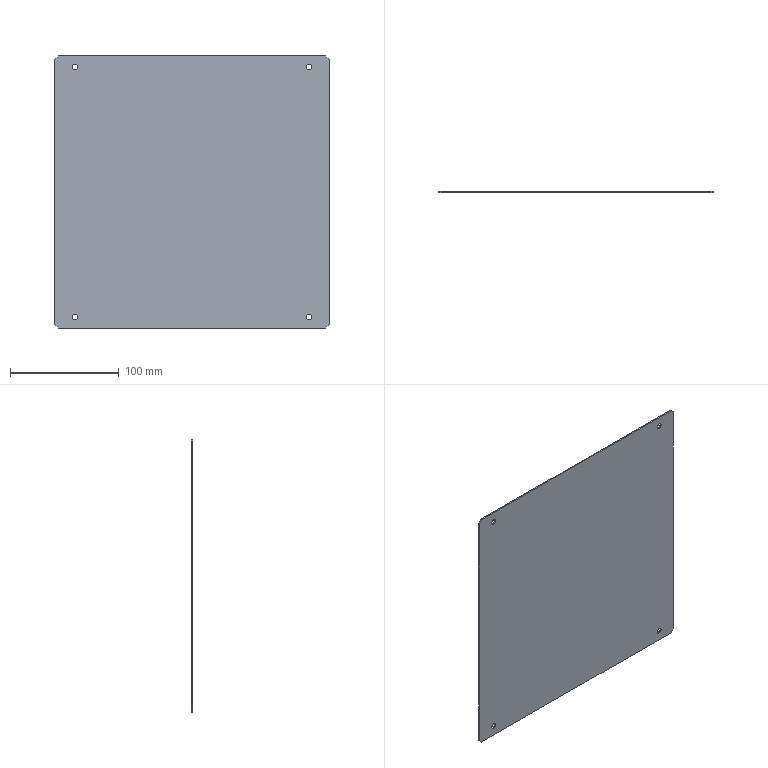Part | STEP file | 1519D3-3_AF0.stp.STEP | 1 solid | 18 faces | box 252 x 1.2 x 250 mm | volume 75484 mm3 | plane 10 | cylinder 8 | commonest cylinder face diameters 5 x8
STEP:
#1=CARTESIAN_POINT('',(105.,0.,-115.));
#2=VERTEX_POINT('',#1);
#3=CARTESIAN_POINT('',(110.,0.,-115.));
#4=VERTEX_POINT('',#3);
#5=CARTESIAN_POINT('',(107.5,0.,-115.));
#6=DIRECTION('',(0.,1.,0.));
#7=DIRECTION('',(-1.,0.,0.));
#8=AXIS2_PLACEMENT_3D('',#5,#6,#7);
#9=CIRCLE('',#8,2.5);
#10=EDGE_CURVE('',#2,#4,#9,.T.);
#11=ORIENTED_EDGE('',*,*,#10,.T.);
#12=CARTESIAN_POINT('',(107.5,0.,-115.));
#13=DIRECTION('',(0.,1.,0.));
#14=DIRECTION('',(1.,0.,0.));
#15=AXIS2_PLACEMENT_3D('',#12,#13,#14);
#16=CIRCLE('',#15,2.5);
#17=EDGE_CURVE('',#4,#2,#16,.T.);
#18=ORIENTED_EDGE('',*,*,#17,.T.);
#19=EDGE_LOOP('',(#11,#18));
#20=FACE_BOUND('',#19,.T.);
#21=CARTESIAN_POINT('',(105.,0.,115.));
#22=VERTEX_POINT('',#21);
#23=CARTESIAN_POINT('',(110.,0.,115.));
#24=VERTEX_POINT('',#23);
#25=CARTESIAN_POINT('',(107.5,0.,115.));
#26=DIRECTION('',(0.,1.,0.));
#27=DIRECTION('',(-1.,0.,0.));
#28=AXIS2_PLACEMENT_3D('',#25,#26,#27);
#29=CIRCLE('',#28,2.5);
#30=EDGE_CURVE('',#22,#24,#29,.T.);
#31=ORIENTED_EDGE('',*,*,#30,.T.);
#32=CARTESIAN_POINT('',(107.5,0.,115.));
#33=DIRECTION('',(0.,1.,0.));
#34=DIRECTION('',(1.,0.,0.));
#35=AXIS2_PLACEMENT_3D('',#32,#33,#34);
#36=CIRCLE('',#35,2.5);
#37=EDGE_CURVE('',#24,#22,#36,.T.);
#38=ORIENTED_EDGE('',*,*,#37,.T.);
#39=EDGE_LOOP('',(#31,#38));
#40=FACE_BOUND('',#39,.T.);
#41=CARTESIAN_POINT('',(-110.,0.,115.));
#42=VERTEX_POINT('',#41);
#43=CARTESIAN_POINT('',(-105.,0.,115.));
#44=VERTEX_POINT('',#43);
#45=CARTESIAN_POINT('',(-107.5,0.,115.));
#46=DIRECTION('',(0.,1.,0.));
#47=DIRECTION('',(-1.,0.,0.));
#48=AXIS2_PLACEMENT_3D('',#45,#46,#47);
#49=CIRCLE('',#48,2.5);
#50=EDGE_CURVE('',#42,#44,#49,.T.);
#51=ORIENTED_EDGE('',*,*,#50,.T.);
#52=CARTESIAN_POINT('',(-107.5,0.,115.));
#53=DIRECTION('',(0.,1.,0.));
#54=DIRECTION('',(1.,0.,0.));
#55=AXIS2_PLACEMENT_3D('',#52,#53,#54);
#56=CIRCLE('',#55,2.5);
#57=EDGE_CURVE('',#44,#42,#56,.T.);
#58=ORIENTED_EDGE('',*,*,#57,.T.);
#59=EDGE_LOOP('',(#51,#58));
#60=FACE_BOUND('',#59,.T.);
#61=CARTESIAN_POINT('',(-110.,0.,-115.));
#62=VERTEX_POINT('',#61);
#63=CARTESIAN_POINT('',(-105.,0.,-115.));
#64=VERTEX_POINT('',#63);
#65=CARTESIAN_POINT('',(-107.5,0.,-115.));
#66=DIRECTION('',(0.,1.,0.));
#67=DIRECTION('',(-1.,0.,0.));
#68=AXIS2_PLACEMENT_3D('',#65,#66,#67);
#69=CIRCLE('',#68,2.5);
#70=EDGE_CURVE('',#62,#64,#69,.T.);
#71=ORIENTED_EDGE('',*,*,#70,.T.);
#72=CARTESIAN_POINT('',(-107.5,0.,-115.));
#73=DIRECTION('',(0.,1.,0.));
#74=DIRECTION('',(1.,0.,0.));
#75=AXIS2_PLACEMENT_3D('',#72,#73,#74);
#76=CIRCLE('',#75,2.5);
#77=EDGE_CURVE('',#64,#62,#76,.T.);
#78=ORIENTED_EDGE('',*,*,#77,.T.);
#79=EDGE_LOOP('',(#71,#78));
#80=FACE_BOUND('',#79,.T.);
#81=CARTESIAN_POINT('',(123.,0.,-125.));
#82=VERTEX_POINT('',#81);
#83=CARTESIAN_POINT('',(-123.,0.,-125.));
#84=VERTEX_POINT('',#83);
#85=CARTESIAN_POINT('',(123.,0.,-125.));
#86=DIRECTION('',(-1.,0.,0.));
#87=VECTOR('',#86,1000.);
#88=LINE('',#85,#87);
#89=EDGE_CURVE('',#82,#84,#88,.T.);
#90=ORIENTED_EDGE('',*,*,#89,.F.);
#91=CARTESIAN_POINT('',(126.,0.,-122.));
#92=VERTEX_POINT('',#91);
#93=CARTESIAN_POINT('',(123.,0.,-125.));
#94=DIRECTION('',(0.7071,0.,0.7071));
#95=VECTOR('',#94,1000.);
#96=LINE('',#93,#95);
#97=EDGE_CURVE('',#82,#92,#96,.T.);
#98=ORIENTED_EDGE('',*,*,#97,.T.);
#99=CARTESIAN_POINT('',(126.,0.,122.));
#100=VERTEX_POINT('',#99);
#101=CARTESIAN_POINT('',(126.,0.,122.));
#102=DIRECTION('',(0.,0.,-1.));
#103=VECTOR('',#102,1000.);
#104=LINE('',#101,#103);
#105=EDGE_CURVE('',#100,#92,#104,.T.);
#106=ORIENTED_EDGE('',*,*,#105,.F.);
#107=CARTESIAN_POINT('',(123.,0.,125.));
#108=VERTEX_POINT('',#107);
#109=CARTESIAN_POINT('',(126.,0.,122.));
#110=DIRECTION('',(-0.7071,0.,0.7071));
#111=VECTOR('',#110,1000.);
#112=LINE('',#109,#111);
#113=EDGE_CURVE('',#100,#108,#112,.T.);
#114=ORIENTED_EDGE('',*,*,#113,.T.);
#115=CARTESIAN_POINT('',(-123.,0.,125.));
#116=VERTEX_POINT('',#115);
#117=CARTESIAN_POINT('',(-123.,0.,125.));
#118=DIRECTION('',(1.,0.,0.));
#119=VECTOR('',#118,1000.);
#120=LINE('',#117,#119);
#121=EDGE_CURVE('',#116,#108,#120,.T.);
#122=ORIENTED_EDGE('',*,*,#121,.F.);
#123=CARTESIAN_POINT('',(-126.,0.,122.));
#124=VERTEX_POINT('',#123);
#125=CARTESIAN_POINT('',(-123.,0.,125.));
#126=DIRECTION('',(-0.7071,0.,-0.7071));
#127=VECTOR('',#126,1000.);
#128=LINE('',#125,#127);
#129=EDGE_CURVE('',#116,#124,#128,.T.);
#130=ORIENTED_EDGE('',*,*,#129,.T.);
#131=CARTESIAN_POINT('',(-126.,0.,-122.));
#132=VERTEX_POINT('',#131);
#133=CARTESIAN_POINT('',(-126.,0.,-122.));
#134=DIRECTION('',(0.,0.,1.));
#135=VECTOR('',#134,1000.);
#136=LINE('',#133,#135);
#137=EDGE_CURVE('',#132,#124,#136,.T.);
#138=ORIENTED_EDGE('',*,*,#137,.F.);
#139=CARTESIAN_POINT('',(-126.,0.,-122.));
#140=DIRECTION('',(0.7071,0.,-0.7071));
#141=VECTOR('',#140,1000.);
#142=LINE('',#139,#141);
#143=EDGE_CURVE('',#132,#84,#142,.T.);
#144=ORIENTED_EDGE('',*,*,#143,.T.);
#145=EDGE_LOOP('',(#90,#98,#106,#114,#122,#130,#138,#144));
#146=FACE_OUTER_BOUND('',#145,.T.);
#147=CARTESIAN_POINT('',(0.,0.,0.));
#148=DIRECTION('',(0.,1.,0.));
#149=DIRECTION('',(1.,0.,0.));
#150=AXIS2_PLACEMENT_3D('',#147,#148,#149);
#151=PLANE('',#150);
#152=ADVANCED_FACE('',(#20,#40,#60,#80,#146),#151,.F.);
#153=CARTESIAN_POINT('',(-105.,1.2,-115.));
#154=VERTEX_POINT('',#153);
#155=CARTESIAN_POINT('',(-105.,1.2,-115.));
#156=DIRECTION('',(0.,-1.,0.));
#157=VECTOR('',#156,1000.);
#158=LINE('',#155,#157);
#159=EDGE_CURVE('',#154,#64,#158,.T.);
#160=ORIENTED_EDGE('',*,*,#159,.F.);
#161=CARTESIAN_POINT('',(-110.,1.2,-115.));
#162=VERTEX_POINT('',#161);
#163=CARTESIAN_POINT('',(-107.5,1.2,-115.));
#164=DIRECTION('',(0.,1.,0.));
#165=DIRECTION('',(1.,0.,0.));
#166=AXIS2_PLACEMENT_3D('',#163,#164,#165);
#167=CIRCLE('',#166,2.5);
#168=EDGE_CURVE('',#154,#162,#167,.T.);
#169=ORIENTED_EDGE('',*,*,#168,.T.);
#170=CARTESIAN_POINT('',(-110.,1.2,-115.));
#171=DIRECTION('',(0.,-1.,0.));
#172=VECTOR('',#171,1000.);
#173=LINE('',#170,#172);
#174=EDGE_CURVE('',#162,#62,#173,.T.);
#175=ORIENTED_EDGE('',*,*,#174,.T.);
#176=ORIENTED_EDGE('',*,*,#77,.F.);
#177=EDGE_LOOP('',(#160,#169,#175,#176));
#178=FACE_OUTER_BOUND('',#177,.T.);
#179=CARTESIAN_POINT('',(-107.5,1.2,-115.));
#180=DIRECTION('',(0.,1.,0.));
#181=DIRECTION('',(1.,0.,0.));
#182=AXIS2_PLACEMENT_3D('',#179,#180,#181);
#183=CYLINDRICAL_SURFACE('',#182,2.5);
#184=ADVANCED_FACE('',(#178),#183,.F.);
#185=ORIENTED_EDGE('',*,*,#174,.F.);
#186=CARTESIAN_POINT('',(-107.5,1.2,-115.));
#187=DIRECTION('',(0.,1.,0.));
#188=DIRECTION('',(-1.,0.,0.));
#189=AXIS2_PLACEMENT_3D('',#186,#187,#188);
#190=CIRCLE('',#189,2.5);
#191=EDGE_CURVE('',#162,#154,#190,.T.);
#192=ORIENTED_EDGE('',*,*,#191,.T.);
#193=ORIENTED_EDGE('',*,*,#159,.T.);
#194=ORIENTED_EDGE('',*,*,#70,.F.);
#195=EDGE_LOOP('',(#185,#192,#193,#194));
#196=FACE_OUTER_BOUND('',#195,.T.);
#197=CARTESIAN_POINT('',(-107.5,1.2,-115.));
#198=DIRECTION('',(0.,1.,0.));
#199=DIRECTION('',(1.,0.,0.));
#200=AXIS2_PLACEMENT_3D('',#197,#198,#199);
#201=CYLINDRICAL_SURFACE('',#200,2.5);
#202=ADVANCED_FACE('',(#196),#201,.F.);
#203=CARTESIAN_POINT('',(105.,1.2,-115.));
#204=VERTEX_POINT('',#203);
#205=CARTESIAN_POINT('',(110.,1.2,-115.));
#206=VERTEX_POINT('',#205);
#207=CARTESIAN_POINT('',(107.5,1.2,-115.));
#208=DIRECTION('',(0.,1.,0.));
#209=DIRECTION('',(-1.,0.,0.));
#210=AXIS2_PLACEMENT_3D('',#207,#208,#209);
#211=CIRCLE('',#210,2.5);
#212=EDGE_CURVE('',#204,#206,#211,.T.);
#213=ORIENTED_EDGE('',*,*,#212,.F.);
#214=CARTESIAN_POINT('',(107.5,1.2,-115.));
#215=DIRECTION('',(0.,1.,0.));
#216=DIRECTION('',(1.,0.,0.));
#217=AXIS2_PLACEMENT_3D('',#214,#215,#216);
#218=CIRCLE('',#217,2.5);
#219=EDGE_CURVE('',#206,#204,#218,.T.);
#220=ORIENTED_EDGE('',*,*,#219,.F.);
#221=EDGE_LOOP('',(#213,#220));
#222=FACE_BOUND('',#221,.T.);
#223=CARTESIAN_POINT('',(105.,1.2,115.));
#224=VERTEX_POINT('',#223);
#225=CARTESIAN_POINT('',(110.,1.2,115.));
#226=VERTEX_POINT('',#225);
#227=CARTESIAN_POINT('',(107.5,1.2,115.));
#228=DIRECTION('',(0.,1.,0.));
#229=DIRECTION('',(-1.,0.,0.));
#230=AXIS2_PLACEMENT_3D('',#227,#228,#229);
#231=CIRCLE('',#230,2.5);
#232=EDGE_CURVE('',#224,#226,#231,.T.);
#233=ORIENTED_EDGE('',*,*,#232,.F.);
#234=CARTESIAN_POINT('',(107.5,1.2,115.));
#235=DIRECTION('',(0.,1.,0.));
#236=DIRECTION('',(1.,0.,0.));
#237=AXIS2_PLACEMENT_3D('',#234,#235,#236);
#238=CIRCLE('',#237,2.5);
#239=EDGE_CURVE('',#226,#224,#238,.T.);
#240=ORIENTED_EDGE('',*,*,#239,.F.);
#241=EDGE_LOOP('',(#233,#240));
#242=FACE_BOUND('',#241,.T.);
#243=CARTESIAN_POINT('',(-110.,1.2,115.));
#244=VERTEX_POINT('',#243);
#245=CARTESIAN_POINT('',(-105.,1.2,115.));
#246=VERTEX_POINT('',#245);
#247=CARTESIAN_POINT('',(-107.5,1.2,115.));
#248=DIRECTION('',(0.,1.,0.));
#249=DIRECTION('',(-1.,0.,0.));
#250=AXIS2_PLACEMENT_3D('',#247,#248,#249);
#251=CIRCLE('',#250,2.5);
#252=EDGE_CURVE('',#244,#246,#251,.T.);
#253=ORIENTED_EDGE('',*,*,#252,.F.);
#254=CARTESIAN_POINT('',(-107.5,1.2,115.));
#255=DIRECTION('',(0.,1.,0.));
#256=DIRECTION('',(1.,0.,0.));
#257=AXIS2_PLACEMENT_3D('',#254,#255,#256);
#258=CIRCLE('',#257,2.5);
#259=EDGE_CURVE('',#246,#244,#258,.T.);
#260=ORIENTED_EDGE('',*,*,#259,.F.);
#261=EDGE_LOOP('',(#253,#260));
#262=FACE_BOUND('',#261,.T.);
#263=ORIENTED_EDGE('',*,*,#191,.F.);
#264=ORIENTED_EDGE('',*,*,#168,.F.);
#265=EDGE_LOOP('',(#263,#264));
#266=FACE_BOUND('',#265,.T.);
#267=CARTESIAN_POINT('',(-126.,1.2,-122.));
#268=VERTEX_POINT('',#267);
#269=CARTESIAN_POINT('',(-126.,1.2,122.));
#270=VERTEX_POINT('',#269);
#271=CARTESIAN_POINT('',(-126.,1.2,-122.));
#272=DIRECTION('',(0.,0.,1.));
#273=VECTOR('',#272,1000.);
#274=LINE('',#271,#273);
#275=EDGE_CURVE('',#268,#270,#274,.T.);
#276=ORIENTED_EDGE('',*,*,#275,.T.);
#277=CARTESIAN_POINT('',(-123.,1.2,125.));
#278=VERTEX_POINT('',#277);
#279=CARTESIAN_POINT('',(-126.,1.2,122.));
#280=DIRECTION('',(0.7071,0.,0.7071));
#281=VECTOR('',#280,1000.);
#282=LINE('',#279,#281);
#283=EDGE_CURVE('',#270,#278,#282,.T.);
#284=ORIENTED_EDGE('',*,*,#283,.T.);
#285=CARTESIAN_POINT('',(123.,1.2,125.));
#286=VERTEX_POINT('',#285);
#287=CARTESIAN_POINT('',(-123.,1.2,125.));
#288=DIRECTION('',(1.,0.,0.));
#289=VECTOR('',#288,1000.);
#290=LINE('',#287,#289);
#291=EDGE_CURVE('',#278,#286,#290,.T.);
#292=ORIENTED_EDGE('',*,*,#291,.T.);
#293=CARTESIAN_POINT('',(126.,1.2,122.));
#294=VERTEX_POINT('',#293);
#295=CARTESIAN_POINT('',(123.,1.2,125.));
#296=DIRECTION('',(0.7071,0.,-0.7071));
#297=VECTOR('',#296,1000.);
#298=LINE('',#295,#297);
#299=EDGE_CURVE('',#286,#294,#298,.T.);
#300=ORIENTED_EDGE('',*,*,#299,.T.);
#301=CARTESIAN_POINT('',(126.,1.2,-122.));
#302=VERTEX_POINT('',#301);
#303=CARTESIAN_POINT('',(126.,1.2,122.));
#304=DIRECTION('',(0.,0.,-1.));
#305=VECTOR('',#304,1000.);
#306=LINE('',#303,#305);
#307=EDGE_CURVE('',#294,#302,#306,.T.);
#308=ORIENTED_EDGE('',*,*,#307,.T.);
#309=CARTESIAN_POINT('',(123.,1.2,-125.));
#310=VERTEX_POINT('',#309);
#311=CARTESIAN_POINT('',(126.,1.2,-122.));
#312=DIRECTION('',(-0.7071,0.,-0.7071));
#313=VECTOR('',#312,1000.);
#314=LINE('',#311,#313);
#315=EDGE_CURVE('',#302,#310,#314,.T.);
#316=ORIENTED_EDGE('',*,*,#315,.T.);
#317=CARTESIAN_POINT('',(-123.,1.2,-125.));
#318=VERTEX_POINT('',#317);
#319=CARTESIAN_POINT('',(123.,1.2,-125.));
#320=DIRECTION('',(-1.,0.,0.));
#321=VECTOR('',#320,1000.);
#322=LINE('',#319,#321);
#323=EDGE_CURVE('',#310,#318,#322,.T.);
#324=ORIENTED_EDGE('',*,*,#323,.T.);
#325=CARTESIAN_POINT('',(-123.,1.2,-125.));
#326=DIRECTION('',(-0.7071,0.,0.7071));
#327=VECTOR('',#326,1000.);
#328=LINE('',#325,#327);
#329=EDGE_CURVE('',#318,#268,#328,.T.);
#330=ORIENTED_EDGE('',*,*,#329,.T.);
#331=EDGE_LOOP('',(#276,#284,#292,#300,#308,#316,#324,#330));
#332=FACE_OUTER_BOUND('',#331,.T.);
#333=CARTESIAN_POINT('',(0.,1.2,0.));
#334=DIRECTION('',(0.,1.,0.));
#335=DIRECTION('',(1.,0.,0.));
#336=AXIS2_PLACEMENT_3D('',#333,#334,#335);
#337=PLANE('',#336);
#338=ADVANCED_FACE('',(#222,#242,#262,#266,#332),#337,.T.);
#339=CARTESIAN_POINT('',(110.,1.2,-115.));
#340=DIRECTION('',(0.,-1.,0.));
#341=VECTOR('',#340,1000.);
#342=LINE('',#339,#341);
#343=EDGE_CURVE('',#206,#4,#342,.T.);
#344=ORIENTED_EDGE('',*,*,#343,.F.);
#345=ORIENTED_EDGE('',*,*,#219,.T.);
#346=CARTESIAN_POINT('',(105.,1.2,-115.));
#347=DIRECTION('',(0.,-1.,0.));
#348=VECTOR('',#347,1000.);
#349=LINE('',#346,#348);
#350=EDGE_CURVE('',#204,#2,#349,.T.);
#351=ORIENTED_EDGE('',*,*,#350,.T.);
#352=ORIENTED_EDGE('',*,*,#17,.F.);
#353=EDGE_LOOP('',(#344,#345,#351,#352));
#354=FACE_OUTER_BOUND('',#353,.T.);
#355=CARTESIAN_POINT('',(107.5,1.2,-115.));
#356=DIRECTION('',(0.,1.,0.));
#357=DIRECTION('',(1.,0.,0.));
#358=AXIS2_PLACEMENT_3D('',#355,#356,#357);
#359=CYLINDRICAL_SURFACE('',#358,2.5);
#360=ADVANCED_FACE('',(#354),#359,.F.);
#361=ORIENTED_EDGE('',*,*,#350,.F.);
#362=ORIENTED_EDGE('',*,*,#212,.T.);
#363=ORIENTED_EDGE('',*,*,#343,.T.);
#364=ORIENTED_EDGE('',*,*,#10,.F.);
#365=EDGE_LOOP('',(#361,#362,#363,#364));
#366=FACE_OUTER_BOUND('',#365,.T.);
#367=CARTESIAN_POINT('',(107.5,1.2,-115.));
#368=DIRECTION('',(0.,1.,0.));
#369=DIRECTION('',(1.,0.,0.));
#370=AXIS2_PLACEMENT_3D('',#367,#368,#369);
#371=CYLINDRICAL_SURFACE('',#370,2.5);
#372=ADVANCED_FACE('',(#366),#371,.F.);
#373=CARTESIAN_POINT('',(110.,1.2,115.));
#374=DIRECTION('',(0.,-1.,0.));
#375=VECTOR('',#374,1000.);
#376=LINE('',#373,#375);
#377=EDGE_CURVE('',#226,#24,#376,.T.);
#378=ORIENTED_EDGE('',*,*,#377,.F.);
#379=ORIENTED_EDGE('',*,*,#239,.T.);
#380=CARTESIAN_POINT('',(105.,1.2,115.));
#381=DIRECTION('',(0.,-1.,0.));
#382=VECTOR('',#381,1000.);
#383=LINE('',#380,#382);
#384=EDGE_CURVE('',#224,#22,#383,.T.);
#385=ORIENTED_EDGE('',*,*,#384,.T.);
#386=ORIENTED_EDGE('',*,*,#37,.F.);
#387=EDGE_LOOP('',(#378,#379,#385,#386));
#388=FACE_OUTER_BOUND('',#387,.T.);
#389=CARTESIAN_POINT('',(107.5,1.2,115.));
#390=DIRECTION('',(0.,1.,0.));
#391=DIRECTION('',(1.,0.,0.));
#392=AXIS2_PLACEMENT_3D('',#389,#390,#391);
#393=CYLINDRICAL_SURFACE('',#392,2.5);
#394=ADVANCED_FACE('',(#388),#393,.F.);
#395=ORIENTED_EDGE('',*,*,#384,.F.);
#396=ORIENTED_EDGE('',*,*,#232,.T.);
#397=ORIENTED_EDGE('',*,*,#377,.T.);
#398=ORIENTED_EDGE('',*,*,#30,.F.);
#399=EDGE_LOOP('',(#395,#396,#397,#398));
#400=FACE_OUTER_BOUND('',#399,.T.);
#401=CARTESIAN_POINT('',(107.5,1.2,115.));
#402=DIRECTION('',(0.,1.,0.));
#403=DIRECTION('',(1.,0.,0.));
#404=AXIS2_PLACEMENT_3D('',#401,#402,#403);
#405=CYLINDRICAL_SURFACE('',#404,2.5);
#406=ADVANCED_FACE('',(#400),#405,.F.);
#407=CARTESIAN_POINT('',(-105.,1.2,115.));
#408=DIRECTION('',(0.,-1.,0.));
#409=VECTOR('',#408,1000.);
#410=LINE('',#407,#409);
#411=EDGE_CURVE('',#246,#44,#410,.T.);
#412=ORIENTED_EDGE('',*,*,#411,.F.);
#413=ORIENTED_EDGE('',*,*,#259,.T.);
#414=CARTESIAN_POINT('',(-110.,1.2,115.));
#415=DIRECTION('',(0.,-1.,0.));
#416=VECTOR('',#415,1000.);
#417=LINE('',#414,#416);
#418=EDGE_CURVE('',#244,#42,#417,.T.);
#419=ORIENTED_EDGE('',*,*,#418,.T.);
#420=ORIENTED_EDGE('',*,*,#57,.F.);
#421=EDGE_LOOP('',(#412,#413,#419,#420));
#422=FACE_OUTER_BOUND('',#421,.T.);
#423=CARTESIAN_POINT('',(-107.5,1.2,115.));
#424=DIRECTION('',(0.,1.,0.));
#425=DIRECTION('',(1.,0.,0.));
#426=AXIS2_PLACEMENT_3D('',#423,#424,#425);
#427=CYLINDRICAL_SURFACE('',#426,2.5);
#428=ADVANCED_FACE('',(#422),#427,.F.);
#429=ORIENTED_EDGE('',*,*,#418,.F.);
#430=ORIENTED_EDGE('',*,*,#252,.T.);
#431=ORIENTED_EDGE('',*,*,#411,.T.);
#432=ORIENTED_EDGE('',*,*,#50,.F.);
#433=EDGE_LOOP('',(#429,#430,#431,#432));
#434=FACE_OUTER_BOUND('',#433,.T.);
#435=CARTESIAN_POINT('',(-107.5,1.2,115.));
#436=DIRECTION('',(0.,1.,0.));
#437=DIRECTION('',(1.,0.,0.));
#438=AXIS2_PLACEMENT_3D('',#435,#436,#437);
#439=CYLINDRICAL_SURFACE('',#438,2.5);
#440=ADVANCED_FACE('',(#434),#439,.F.);
#441=CARTESIAN_POINT('',(-126.,1.2,-122.));
#442=DIRECTION('',(0.,-1.,0.));
#443=VECTOR('',#442,1000.);
#444=LINE('',#441,#443);
#445=EDGE_CURVE('',#268,#132,#444,.T.);
#446=ORIENTED_EDGE('',*,*,#445,.F.);
#447=ORIENTED_EDGE('',*,*,#329,.F.);
#448=CARTESIAN_POINT('',(-123.,1.2,-125.));
#449=DIRECTION('',(0.,-1.,0.));
#450=VECTOR('',#449,1000.);
#451=LINE('',#448,#450);
#452=EDGE_CURVE('',#318,#84,#451,.T.);
#453=ORIENTED_EDGE('',*,*,#452,.T.);
#454=ORIENTED_EDGE('',*,*,#143,.F.);
#455=EDGE_LOOP('',(#446,#447,#453,#454));
#456=FACE_OUTER_BOUND('',#455,.T.);
#457=CARTESIAN_POINT('',(-124.5,0.6,-123.5));
#458=DIRECTION('',(-0.7071,0.,-0.7071));
#459=DIRECTION('',(-0.7071,0.,0.7071));
#460=AXIS2_PLACEMENT_3D('',#457,#458,#459);
#461=PLANE('',#460);
#462=ADVANCED_FACE('',(#456),#461,.T.);
#463=ORIENTED_EDGE('',*,*,#323,.F.);
#464=CARTESIAN_POINT('',(123.,1.2,-125.));
#465=DIRECTION('',(0.,-1.,0.));
#466=VECTOR('',#465,1000.);
#467=LINE('',#464,#466);
#468=EDGE_CURVE('',#310,#82,#467,.T.);
#469=ORIENTED_EDGE('',*,*,#468,.T.);
#470=ORIENTED_EDGE('',*,*,#89,.T.);
#471=ORIENTED_EDGE('',*,*,#452,.F.);
#472=EDGE_LOOP('',(#463,#469,#470,#471));
#473=FACE_OUTER_BOUND('',#472,.T.);
#474=CARTESIAN_POINT('',(126.,0.,-125.));
#475=DIRECTION('',(0.,0.,-1.));
#476=DIRECTION('',(0.,-1.,0.));
#477=AXIS2_PLACEMENT_3D('',#474,#475,#476);
#478=PLANE('',#477);
#479=ADVANCED_FACE('',(#473),#478,.T.);
#480=ORIENTED_EDGE('',*,*,#468,.F.);
#481=ORIENTED_EDGE('',*,*,#315,.F.);
#482=CARTESIAN_POINT('',(126.,1.2,-122.));
#483=DIRECTION('',(0.,-1.,0.));
#484=VECTOR('',#483,1000.);
#485=LINE('',#482,#484);
#486=EDGE_CURVE('',#302,#92,#485,.T.);
#487=ORIENTED_EDGE('',*,*,#486,.T.);
#488=ORIENTED_EDGE('',*,*,#97,.F.);
#489=EDGE_LOOP('',(#480,#481,#487,#488));
#490=FACE_OUTER_BOUND('',#489,.T.);
#491=CARTESIAN_POINT('',(124.5,0.6,-123.5));
#492=DIRECTION('',(0.7071,0.,-0.7071));
#493=DIRECTION('',(0.,-1.,0.));
#494=AXIS2_PLACEMENT_3D('',#491,#492,#493);
#495=PLANE('',#494);
#496=ADVANCED_FACE('',(#490),#495,.T.);
#497=ORIENTED_EDGE('',*,*,#307,.F.);
#498=CARTESIAN_POINT('',(126.,1.2,122.));
#499=DIRECTION('',(0.,-1.,0.));
#500=VECTOR('',#499,1000.);
#501=LINE('',#498,#500);
#502=EDGE_CURVE('',#294,#100,#501,.T.);
#503=ORIENTED_EDGE('',*,*,#502,.T.);
#504=ORIENTED_EDGE('',*,*,#105,.T.);
#505=ORIENTED_EDGE('',*,*,#486,.F.);
#506=EDGE_LOOP('',(#497,#503,#504,#505));
#507=FACE_OUTER_BOUND('',#506,.T.);
#508=CARTESIAN_POINT('',(126.,0.,125.));
#509=DIRECTION('',(1.,0.,0.));
#510=DIRECTION('',(0.,1.,0.));
#511=AXIS2_PLACEMENT_3D('',#508,#509,#510);
#512=PLANE('',#511);
#513=ADVANCED_FACE('',(#507),#512,.T.);
#514=ORIENTED_EDGE('',*,*,#502,.F.);
#515=ORIENTED_EDGE('',*,*,#299,.F.);
#516=CARTESIAN_POINT('',(123.,1.2,125.));
#517=DIRECTION('',(0.,-1.,0.));
#518=VECTOR('',#517,1000.);
#519=LINE('',#516,#518);
#520=EDGE_CURVE('',#286,#108,#519,.T.);
#521=ORIENTED_EDGE('',*,*,#520,.T.);
#522=ORIENTED_EDGE('',*,*,#113,.F.);
#523=EDGE_LOOP('',(#514,#515,#521,#522));
#524=FACE_OUTER_BOUND('',#523,.T.);
#525=CARTESIAN_POINT('',(124.5,0.6,123.5));
#526=DIRECTION('',(0.7071,0.,0.7071));
#527=DIRECTION('',(0.,-1.,0.));
#528=AXIS2_PLACEMENT_3D('',#525,#526,#527);
#529=PLANE('',#528);
#530=ADVANCED_FACE('',(#524),#529,.T.);
#531=ORIENTED_EDGE('',*,*,#121,.T.);
#532=ORIENTED_EDGE('',*,*,#520,.F.);
#533=ORIENTED_EDGE('',*,*,#291,.F.);
#534=CARTESIAN_POINT('',(-123.,1.2,125.));
#535=DIRECTION('',(0.,-1.,0.));
#536=VECTOR('',#535,1000.);
#537=LINE('',#534,#536);
#538=EDGE_CURVE('',#278,#116,#537,.T.);
#539=ORIENTED_EDGE('',*,*,#538,.T.);
#540=EDGE_LOOP('',(#531,#532,#533,#539));
#541=FACE_OUTER_BOUND('',#540,.T.);
#542=CARTESIAN_POINT('',(-126.,0.,125.));
#543=DIRECTION('',(0.,0.,1.));
#544=DIRECTION('',(1.,0.,0.));
#545=AXIS2_PLACEMENT_3D('',#542,#543,#544);
#546=PLANE('',#545);
#547=ADVANCED_FACE('',(#541),#546,.T.);
#548=ORIENTED_EDGE('',*,*,#538,.F.);
#549=ORIENTED_EDGE('',*,*,#283,.F.);
#550=CARTESIAN_POINT('',(-126.,1.2,122.));
#551=DIRECTION('',(0.,-1.,0.));
#552=VECTOR('',#551,1000.);
#553=LINE('',#550,#552);
#554=EDGE_CURVE('',#270,#124,#553,.T.);
#555=ORIENTED_EDGE('',*,*,#554,.T.);
#556=ORIENTED_EDGE('',*,*,#129,.F.);
#557=EDGE_LOOP('',(#548,#549,#555,#556));
#558=FACE_OUTER_BOUND('',#557,.T.);
#559=CARTESIAN_POINT('',(-124.5,0.6,123.5));
#560=DIRECTION('',(-0.7071,0.,0.7071));
#561=DIRECTION('',(0.,1.,0.));
#562=AXIS2_PLACEMENT_3D('',#559,#560,#561);
#563=PLANE('',#562);
#564=ADVANCED_FACE('',(#558),#563,.T.);
#565=ORIENTED_EDGE('',*,*,#137,.T.);
#566=ORIENTED_EDGE('',*,*,#554,.F.);
#567=ORIENTED_EDGE('',*,*,#275,.F.);
#568=ORIENTED_EDGE('',*,*,#445,.T.);
#569=EDGE_LOOP('',(#565,#566,#567,#568));
#570=FACE_OUTER_BOUND('',#569,.T.);
#571=CARTESIAN_POINT('',(-126.,0.,-125.));
#572=DIRECTION('',(-1.,0.,0.));
#573=DIRECTION('',(0.,0.,1.));
#574=AXIS2_PLACEMENT_3D('',#571,#572,#573);
#575=PLANE('',#574);
#576=ADVANCED_FACE('',(#570),#575,.T.);
#577=CLOSED_SHELL('',(#152,#184,#202,#338,#360,#372,#394,#406,#428,#440,#462,#479,#496,#513,#530,#547,#564,#576));
#578=MANIFOLD_SOLID_BREP('',#577);
#579=CARTESIAN_POINT('',(0.,0.,0.));
#580=DIRECTION('',(0.,0.,1.));
#581=DIRECTION('',(1.,0.,0.));
#582=AXIS2_PLACEMENT_3D('',#579,#580,#581);
#583=(LENGTH_UNIT()NAMED_UNIT(*)SI_UNIT(.MILLI.,.METRE.));
#584=UNCERTAINTY_MEASURE_WITH_UNIT(LENGTH_MEASURE(0.00001),#583,'','');
#585=(NAMED_UNIT(*)PLANE_ANGLE_UNIT()SI_UNIT($,.RADIAN.));
#586=(NAMED_UNIT(*)SI_UNIT($,.STERADIAN.)SOLID_ANGLE_UNIT());
#587=(GEOMETRIC_REPRESENTATION_CONTEXT(3)GLOBAL_UNCERTAINTY_ASSIGNED_CONTEXT((#584))GLOBAL_UNIT_ASSIGNED_CONTEXT((#583,#585,#586))REPRESENTATION_CONTEXT('',''));
#588=ADVANCED_BREP_SHAPE_REPRESENTATION('',(#578,#582),#587);